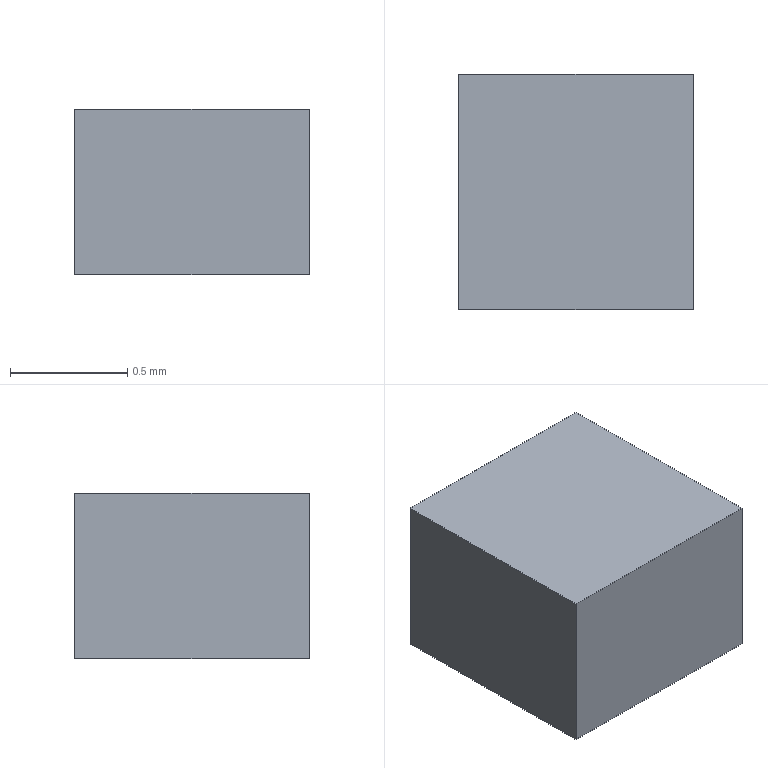Part | Creo | 1 solid | 6 faces | box 1 x 1 x 0.7071 mm | volume 0.7071 mm3 | plane 6
STEP:
#1=CARTESIAN_POINT('',(0.,0.,0.));
#2=DIRECTION('',(0.,0.,1.));
#3=DIRECTION('',(1.,0.,0.));
#4=AXIS2_PLACEMENT_3D('',#1,#2,#3);
#5=CARTESIAN_POINT('',(-0.5,-0.5,0.));
#6=VERTEX_POINT('',#5);
#7=CARTESIAN_POINT('',(0.5,-0.5,0.));
#8=VERTEX_POINT('',#7);
#9=CARTESIAN_POINT('',(-0.5,-0.5,0.));
#10=DIRECTION('',(1.,0.,0.));
#11=VECTOR('',#10,1.);
#12=LINE('',#9,#11);
#13=EDGE_CURVE('',#6,#8,#12,.T.);
#14=ORIENTED_EDGE('',*,*,#13,.T.);
#15=CARTESIAN_POINT('',(0.5,0.5,0.));
#16=VERTEX_POINT('',#15);
#17=CARTESIAN_POINT('',(0.5,-0.5,0.));
#18=DIRECTION('',(0.,1.,0.));
#19=VECTOR('',#18,1.);
#20=LINE('',#17,#19);
#21=EDGE_CURVE('',#8,#16,#20,.T.);
#22=ORIENTED_EDGE('',*,*,#21,.T.);
#23=CARTESIAN_POINT('',(-0.5,0.5,0.));
#24=VERTEX_POINT('',#23);
#25=CARTESIAN_POINT('',(0.5,0.5,0.));
#26=DIRECTION('',(-1.,0.,0.));
#27=VECTOR('',#26,1.);
#28=LINE('',#25,#27);
#29=EDGE_CURVE('',#16,#24,#28,.T.);
#30=ORIENTED_EDGE('',*,*,#29,.T.);
#31=CARTESIAN_POINT('',(-0.5,0.5,0.));
#32=DIRECTION('',(0.,-1.,0.));
#33=VECTOR('',#32,1.);
#34=LINE('',#31,#33);
#35=EDGE_CURVE('',#24,#6,#34,.T.);
#36=ORIENTED_EDGE('',*,*,#35,.T.);
#37=EDGE_LOOP('',(#14,#22,#30,#36));
#38=FACE_OUTER_BOUND('',#37,.F.);
#39=CARTESIAN_POINT('',(0.,0.,0.));
#40=DIRECTION('',(0.,0.,1.));
#41=DIRECTION('',(1.,0.,0.));
#42=AXIS2_PLACEMENT_3D('',#39,#40,#41);
#43=PLANE('',#42);
#44=ADVANCED_FACE('',(#38),#43,.F.);
#45=ORIENTED_EDGE('',*,*,#13,.F.);
#46=CARTESIAN_POINT('',(-0.5,-0.5,0.7071));
#47=VERTEX_POINT('',#46);
#48=CARTESIAN_POINT('',(-0.5,-0.5,0.));
#49=DIRECTION('',(0.,0.,1.));
#50=VECTOR('',#49,0.7071);
#51=LINE('',#48,#50);
#52=EDGE_CURVE('',#6,#47,#51,.T.);
#53=ORIENTED_EDGE('',*,*,#52,.T.);
#54=CARTESIAN_POINT('',(0.5,-0.5,0.7071));
#55=VERTEX_POINT('',#54);
#56=CARTESIAN_POINT('',(-0.5,-0.5,0.7071));
#57=DIRECTION('',(1.,0.,0.));
#58=VECTOR('',#57,1.);
#59=LINE('',#56,#58);
#60=EDGE_CURVE('',#47,#55,#59,.T.);
#61=ORIENTED_EDGE('',*,*,#60,.T.);
#62=CARTESIAN_POINT('',(0.5,-0.5,0.));
#63=DIRECTION('',(0.,0.,1.));
#64=VECTOR('',#63,0.7071);
#65=LINE('',#62,#64);
#66=EDGE_CURVE('',#8,#55,#65,.T.);
#67=ORIENTED_EDGE('',*,*,#66,.F.);
#68=EDGE_LOOP('',(#45,#53,#61,#67));
#69=FACE_OUTER_BOUND('',#68,.F.);
#70=CARTESIAN_POINT('',(-0.5,-0.5,0.));
#71=DIRECTION('',(0.,-1.,0.));
#72=DIRECTION('',(1.,0.,0.));
#73=AXIS2_PLACEMENT_3D('',#70,#71,#72);
#74=PLANE('',#73);
#75=ADVANCED_FACE('',(#69),#74,.T.);
#76=ORIENTED_EDGE('',*,*,#35,.F.);
#77=CARTESIAN_POINT('',(-0.5,0.5,0.7071));
#78=VERTEX_POINT('',#77);
#79=CARTESIAN_POINT('',(-0.5,0.5,0.));
#80=DIRECTION('',(0.,0.,1.));
#81=VECTOR('',#80,0.7071);
#82=LINE('',#79,#81);
#83=EDGE_CURVE('',#24,#78,#82,.T.);
#84=ORIENTED_EDGE('',*,*,#83,.T.);
#85=CARTESIAN_POINT('',(-0.5,0.5,0.7071));
#86=DIRECTION('',(0.,-1.,0.));
#87=VECTOR('',#86,1.);
#88=LINE('',#85,#87);
#89=EDGE_CURVE('',#78,#47,#88,.T.);
#90=ORIENTED_EDGE('',*,*,#89,.T.);
#91=ORIENTED_EDGE('',*,*,#52,.F.);
#92=EDGE_LOOP('',(#76,#84,#90,#91));
#93=FACE_OUTER_BOUND('',#92,.F.);
#94=CARTESIAN_POINT('',(-0.5,0.5,0.));
#95=DIRECTION('',(-1.,0.,0.));
#96=DIRECTION('',(0.,-1.,0.));
#97=AXIS2_PLACEMENT_3D('',#94,#95,#96);
#98=PLANE('',#97);
#99=ADVANCED_FACE('',(#93),#98,.T.);
#100=ORIENTED_EDGE('',*,*,#29,.F.);
#101=CARTESIAN_POINT('',(0.5,0.5,0.7071));
#102=VERTEX_POINT('',#101);
#103=CARTESIAN_POINT('',(0.5,0.5,0.));
#104=DIRECTION('',(0.,0.,1.));
#105=VECTOR('',#104,0.7071);
#106=LINE('',#103,#105);
#107=EDGE_CURVE('',#16,#102,#106,.T.);
#108=ORIENTED_EDGE('',*,*,#107,.T.);
#109=CARTESIAN_POINT('',(0.5,0.5,0.7071));
#110=DIRECTION('',(-1.,0.,0.));
#111=VECTOR('',#110,1.);
#112=LINE('',#109,#111);
#113=EDGE_CURVE('',#102,#78,#112,.T.);
#114=ORIENTED_EDGE('',*,*,#113,.T.);
#115=ORIENTED_EDGE('',*,*,#83,.F.);
#116=EDGE_LOOP('',(#100,#108,#114,#115));
#117=FACE_OUTER_BOUND('',#116,.F.);
#118=CARTESIAN_POINT('',(0.5,0.5,0.));
#119=DIRECTION('',(0.,1.,0.));
#120=DIRECTION('',(-1.,0.,0.));
#121=AXIS2_PLACEMENT_3D('',#118,#119,#120);
#122=PLANE('',#121);
#123=ADVANCED_FACE('',(#117),#122,.T.);
#124=ORIENTED_EDGE('',*,*,#21,.F.);
#125=ORIENTED_EDGE('',*,*,#66,.T.);
#126=CARTESIAN_POINT('',(0.5,-0.5,0.7071));
#127=DIRECTION('',(0.,1.,0.));
#128=VECTOR('',#127,1.);
#129=LINE('',#126,#128);
#130=EDGE_CURVE('',#55,#102,#129,.T.);
#131=ORIENTED_EDGE('',*,*,#130,.T.);
#132=ORIENTED_EDGE('',*,*,#107,.F.);
#133=EDGE_LOOP('',(#124,#125,#131,#132));
#134=FACE_OUTER_BOUND('',#133,.F.);
#135=CARTESIAN_POINT('',(0.5,-0.5,0.));
#136=DIRECTION('',(1.,0.,0.));
#137=DIRECTION('',(0.,1.,0.));
#138=AXIS2_PLACEMENT_3D('',#135,#136,#137);
#139=PLANE('',#138);
#140=ADVANCED_FACE('',(#134),#139,.T.);
#141=ORIENTED_EDGE('',*,*,#60,.F.);
#142=ORIENTED_EDGE('',*,*,#89,.F.);
#143=ORIENTED_EDGE('',*,*,#113,.F.);
#144=ORIENTED_EDGE('',*,*,#130,.F.);
#145=EDGE_LOOP('',(#141,#142,#143,#144));
#146=FACE_OUTER_BOUND('',#145,.F.);
#147=CARTESIAN_POINT('',(0.,0.,0.7071));
#148=DIRECTION('',(0.,0.,1.));
#149=DIRECTION('',(1.,0.,0.));
#150=AXIS2_PLACEMENT_3D('',#147,#148,#149);
#151=PLANE('',#150);
#152=ADVANCED_FACE('',(#146),#151,.T.);
#153=CLOSED_SHELL('',(#44,#75,#99,#123,#140,#152));
#154=MANIFOLD_SOLID_BREP('',#153);
#155=(LENGTH_UNIT()NAMED_UNIT(*)SI_UNIT(.MILLI.,.METRE.));
#156=UNCERTAINTY_MEASURE_WITH_UNIT(LENGTH_MEASURE(0.0001581),#155,'','');
#157=(NAMED_UNIT(*)PLANE_ANGLE_UNIT()SI_UNIT($,.RADIAN.));
#158=PLANE_ANGLE_MEASURE_WITH_UNIT(PLANE_ANGLE_MEASURE(0.01745),#157);
#159=(CONVERSION_BASED_UNIT('DEGREE',#158)NAMED_UNIT(*)PLANE_ANGLE_UNIT());
#160=(NAMED_UNIT(*)SI_UNIT($,.STERADIAN.)SOLID_ANGLE_UNIT());
#161=(GEOMETRIC_REPRESENTATION_CONTEXT(3)GLOBAL_UNCERTAINTY_ASSIGNED_CONTEXT((#156))GLOBAL_UNIT_ASSIGNED_CONTEXT((#155,#159,#160))REPRESENTATION_CONTEXT('',''));
#162=ADVANCED_BREP_SHAPE_REPRESENTATION('',(#4,#154),#161);